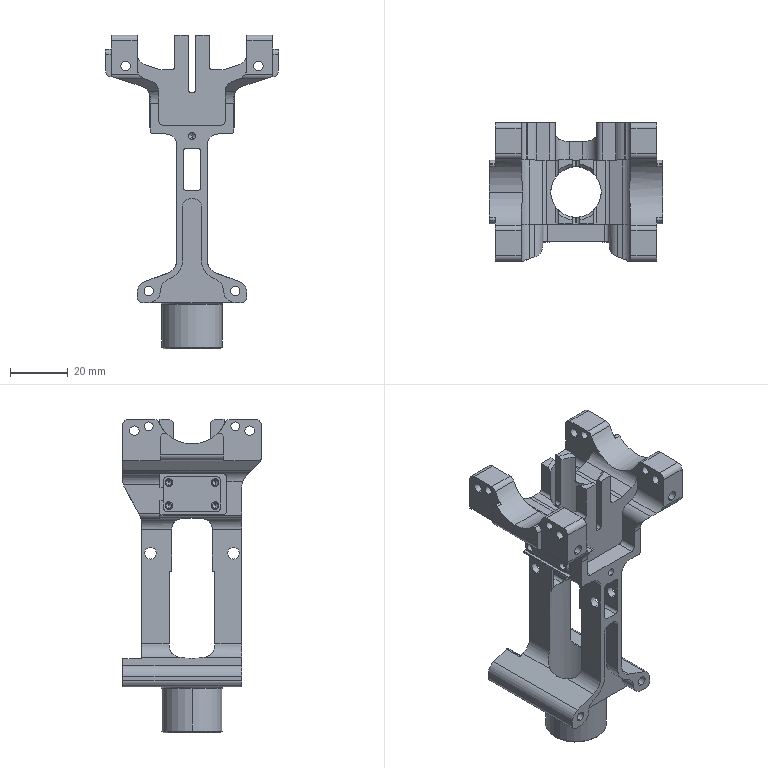Part | SolidWorks | 9 solids | 420 faces | box 60 x 48 x 108.75 mm | volume 36754 mm3 | cylinder 212 | plane 168 | cone 26 | torus 8 | sphere 4 | spline 2 | commonest cylinder face diameters 2 x41 4 x22 8 x18 2.05 x16 2.7 x16 3.3 x16